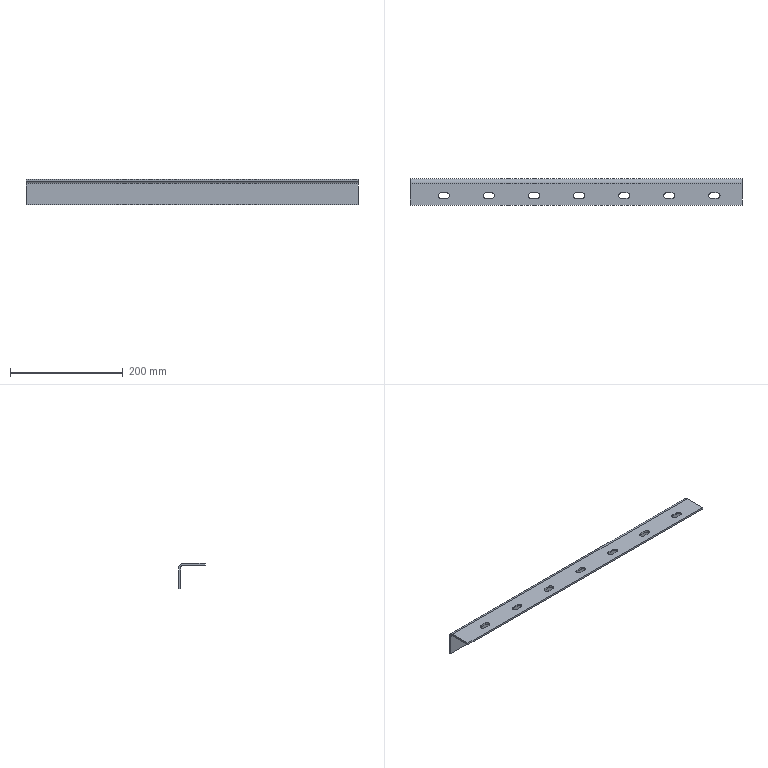Part | SolidWorks | features FlatPattern 1, ICE 1, SMBaseFlange 1, SheetMetal 1 | 1 solid | 49 faces | box 589 x 47 x 45 mm | volume 158032 mm3 | plane 26 | cylinder 23 | commonest cylinder face diameters 10 x22 16.4 x1
STEP:
#1=CARTESIAN_POINT('',(65.,-25.,-3.2));
#2=VERTEX_POINT('',#1);
#3=CARTESIAN_POINT('',(70.,-30.,-3.2));
#4=VERTEX_POINT('',#3);
#5=CARTESIAN_POINT('',(65.,-30.,-3.2));
#6=DIRECTION('',(0.,0.,-1.));
#7=DIRECTION('',(0.,1.,0.));
#8=AXIS2_PLACEMENT_3D('',#5,#6,#7);
#9=CIRCLE('',#8,5.);
#10=EDGE_CURVE('',#2,#4,#9,.T.);
#11=ORIENTED_EDGE('',*,*,#10,.T.);
#12=CARTESIAN_POINT('',(70.,-30.,0.));
#13=VERTEX_POINT('',#12);
#14=CARTESIAN_POINT('',(70.,-30.,-45.));
#15=DIRECTION('',(0.,0.,1.));
#16=VECTOR('',#15,1000.);
#17=LINE('',#14,#16);
#18=EDGE_CURVE('',#4,#13,#17,.T.);
#19=ORIENTED_EDGE('',*,*,#18,.T.);
#20=CARTESIAN_POINT('',(65.,-25.,0.));
#21=VERTEX_POINT('',#20);
#22=CARTESIAN_POINT('',(65.,-30.,0.));
#23=DIRECTION('',(0.,0.,1.));
#24=DIRECTION('',(1.,0.,0.));
#25=AXIS2_PLACEMENT_3D('',#22,#23,#24);
#26=CIRCLE('',#25,5.);
#27=EDGE_CURVE('',#13,#21,#26,.T.);
#28=ORIENTED_EDGE('',*,*,#27,.T.);
#29=CARTESIAN_POINT('',(65.,-25.,-45.));
#30=DIRECTION('',(0.,0.,1.));
#31=VECTOR('',#30,1000.);
#32=LINE('',#29,#31);
#33=EDGE_CURVE('',#2,#21,#32,.T.);
#34=ORIENTED_EDGE('',*,*,#33,.F.);
#35=EDGE_LOOP('',(#11,#19,#28,#34));
#36=FACE_OUTER_BOUND('',#35,.T.);
#37=CARTESIAN_POINT('',(65.,-30.,-45.));
#38=DIRECTION('',(0.,0.,1.));
#39=DIRECTION('',(1.,0.,0.));
#40=AXIS2_PLACEMENT_3D('',#37,#38,#39);
#41=CYLINDRICAL_SURFACE('',#40,5.);
#42=ADVANCED_FACE('',(#36),#41,.F.);
#43=CARTESIAN_POINT('',(145.,-25.,-3.2));
#44=VERTEX_POINT('',#43);
#45=CARTESIAN_POINT('',(150.,-30.,-3.2));
#46=VERTEX_POINT('',#45);
#47=CARTESIAN_POINT('',(145.,-30.,-3.2));
#48=DIRECTION('',(0.,0.,-1.));
#49=DIRECTION('',(0.,1.,0.));
#50=AXIS2_PLACEMENT_3D('',#47,#48,#49);
#51=CIRCLE('',#50,5.);
#52=EDGE_CURVE('',#44,#46,#51,.T.);
#53=ORIENTED_EDGE('',*,*,#52,.T.);
#54=CARTESIAN_POINT('',(150.,-30.,0.));
#55=VERTEX_POINT('',#54);
#56=CARTESIAN_POINT('',(150.,-30.,-45.));
#57=DIRECTION('',(0.,0.,1.));
#58=VECTOR('',#57,1000.);
#59=LINE('',#56,#58);
#60=EDGE_CURVE('',#46,#55,#59,.T.);
#61=ORIENTED_EDGE('',*,*,#60,.T.);
#62=CARTESIAN_POINT('',(145.,-25.,0.));
#63=VERTEX_POINT('',#62);
#64=CARTESIAN_POINT('',(145.,-30.,0.));
#65=DIRECTION('',(0.,0.,1.));
#66=DIRECTION('',(1.,0.,0.));
#67=AXIS2_PLACEMENT_3D('',#64,#65,#66);
#68=CIRCLE('',#67,5.);
#69=EDGE_CURVE('',#55,#63,#68,.T.);
#70=ORIENTED_EDGE('',*,*,#69,.T.);
#71=CARTESIAN_POINT('',(145.,-25.,-45.));
#72=DIRECTION('',(0.,0.,1.));
#73=VECTOR('',#72,1000.);
#74=LINE('',#71,#73);
#75=EDGE_CURVE('',#44,#63,#74,.T.);
#76=ORIENTED_EDGE('',*,*,#75,.F.);
#77=EDGE_LOOP('',(#53,#61,#70,#76));
#78=FACE_OUTER_BOUND('',#77,.T.);
#79=CARTESIAN_POINT('',(145.,-30.,-45.));
#80=DIRECTION('',(0.,0.,1.));
#81=DIRECTION('',(1.,0.,0.));
#82=AXIS2_PLACEMENT_3D('',#79,#80,#81);
#83=CYLINDRICAL_SURFACE('',#82,5.);
#84=ADVANCED_FACE('',(#78),#83,.F.);
#85=CARTESIAN_POINT('',(225.,-25.,-3.2));
#86=VERTEX_POINT('',#85);
#87=CARTESIAN_POINT('',(230.,-30.,-3.2));
#88=VERTEX_POINT('',#87);
#89=CARTESIAN_POINT('',(225.,-30.,-3.2));
#90=DIRECTION('',(0.,0.,-1.));
#91=DIRECTION('',(0.,1.,0.));
#92=AXIS2_PLACEMENT_3D('',#89,#90,#91);
#93=CIRCLE('',#92,5.);
#94=EDGE_CURVE('',#86,#88,#93,.T.);
#95=ORIENTED_EDGE('',*,*,#94,.T.);
#96=CARTESIAN_POINT('',(230.,-30.,0.));
#97=VERTEX_POINT('',#96);
#98=CARTESIAN_POINT('',(230.,-30.,-45.));
#99=DIRECTION('',(0.,0.,1.));
#100=VECTOR('',#99,1000.);
#101=LINE('',#98,#100);
#102=EDGE_CURVE('',#88,#97,#101,.T.);
#103=ORIENTED_EDGE('',*,*,#102,.T.);
#104=CARTESIAN_POINT('',(225.,-25.,0.));
#105=VERTEX_POINT('',#104);
#106=CARTESIAN_POINT('',(225.,-30.,0.));
#107=DIRECTION('',(0.,0.,1.));
#108=DIRECTION('',(1.,0.,0.));
#109=AXIS2_PLACEMENT_3D('',#106,#107,#108);
#110=CIRCLE('',#109,5.);
#111=EDGE_CURVE('',#97,#105,#110,.T.);
#112=ORIENTED_EDGE('',*,*,#111,.T.);
#113=CARTESIAN_POINT('',(225.,-25.,-45.));
#114=DIRECTION('',(0.,0.,1.));
#115=VECTOR('',#114,1000.);
#116=LINE('',#113,#115);
#117=EDGE_CURVE('',#86,#105,#116,.T.);
#118=ORIENTED_EDGE('',*,*,#117,.F.);
#119=EDGE_LOOP('',(#95,#103,#112,#118));
#120=FACE_OUTER_BOUND('',#119,.T.);
#121=CARTESIAN_POINT('',(225.,-30.,-45.));
#122=DIRECTION('',(0.,0.,1.));
#123=DIRECTION('',(1.,0.,0.));
#124=AXIS2_PLACEMENT_3D('',#121,#122,#123);
#125=CYLINDRICAL_SURFACE('',#124,5.);
#126=ADVANCED_FACE('',(#120),#125,.F.);
#127=CARTESIAN_POINT('',(305.,-25.,-3.2));
#128=VERTEX_POINT('',#127);
#129=CARTESIAN_POINT('',(310.,-30.,-3.2));
#130=VERTEX_POINT('',#129);
#131=CARTESIAN_POINT('',(305.,-30.,-3.2));
#132=DIRECTION('',(0.,0.,-1.));
#133=DIRECTION('',(0.,1.,0.));
#134=AXIS2_PLACEMENT_3D('',#131,#132,#133);
#135=CIRCLE('',#134,5.);
#136=EDGE_CURVE('',#128,#130,#135,.T.);
#137=ORIENTED_EDGE('',*,*,#136,.T.);
#138=CARTESIAN_POINT('',(310.,-30.,0.));
#139=VERTEX_POINT('',#138);
#140=CARTESIAN_POINT('',(310.,-30.,-45.));
#141=DIRECTION('',(0.,0.,1.));
#142=VECTOR('',#141,1000.);
#143=LINE('',#140,#142);
#144=EDGE_CURVE('',#130,#139,#143,.T.);
#145=ORIENTED_EDGE('',*,*,#144,.T.);
#146=CARTESIAN_POINT('',(305.,-25.,0.));
#147=VERTEX_POINT('',#146);
#148=CARTESIAN_POINT('',(305.,-30.,0.));
#149=DIRECTION('',(0.,0.,1.));
#150=DIRECTION('',(1.,0.,0.));
#151=AXIS2_PLACEMENT_3D('',#148,#149,#150);
#152=CIRCLE('',#151,5.);
#153=EDGE_CURVE('',#139,#147,#152,.T.);
#154=ORIENTED_EDGE('',*,*,#153,.T.);
#155=CARTESIAN_POINT('',(305.,-25.,-45.));
#156=DIRECTION('',(0.,0.,1.));
#157=VECTOR('',#156,1000.);
#158=LINE('',#155,#157);
#159=EDGE_CURVE('',#128,#147,#158,.T.);
#160=ORIENTED_EDGE('',*,*,#159,.F.);
#161=EDGE_LOOP('',(#137,#145,#154,#160));
#162=FACE_OUTER_BOUND('',#161,.T.);
#163=CARTESIAN_POINT('',(305.,-30.,-45.));
#164=DIRECTION('',(0.,0.,1.));
#165=DIRECTION('',(1.,0.,0.));
#166=AXIS2_PLACEMENT_3D('',#163,#164,#165);
#167=CYLINDRICAL_SURFACE('',#166,5.);
#168=ADVANCED_FACE('',(#162),#167,.F.);
#169=CARTESIAN_POINT('',(385.,-25.,-3.2));
#170=VERTEX_POINT('',#169);
#171=CARTESIAN_POINT('',(390.,-30.,-3.2));
#172=VERTEX_POINT('',#171);
#173=CARTESIAN_POINT('',(385.,-30.,-3.2));
#174=DIRECTION('',(0.,0.,-1.));
#175=DIRECTION('',(0.,1.,0.));
#176=AXIS2_PLACEMENT_3D('',#173,#174,#175);
#177=CIRCLE('',#176,5.);
#178=EDGE_CURVE('',#170,#172,#177,.T.);
#179=ORIENTED_EDGE('',*,*,#178,.T.);
#180=CARTESIAN_POINT('',(390.,-30.,0.));
#181=VERTEX_POINT('',#180);
#182=CARTESIAN_POINT('',(390.,-30.,-45.));
#183=DIRECTION('',(0.,0.,1.));
#184=VECTOR('',#183,1000.);
#185=LINE('',#182,#184);
#186=EDGE_CURVE('',#172,#181,#185,.T.);
#187=ORIENTED_EDGE('',*,*,#186,.T.);
#188=CARTESIAN_POINT('',(385.,-25.,0.));
#189=VERTEX_POINT('',#188);
#190=CARTESIAN_POINT('',(385.,-30.,0.));
#191=DIRECTION('',(0.,0.,1.));
#192=DIRECTION('',(1.,0.,0.));
#193=AXIS2_PLACEMENT_3D('',#190,#191,#192);
#194=CIRCLE('',#193,5.);
#195=EDGE_CURVE('',#181,#189,#194,.T.);
#196=ORIENTED_EDGE('',*,*,#195,.T.);
#197=CARTESIAN_POINT('',(385.,-25.,-45.));
#198=DIRECTION('',(0.,0.,1.));
#199=VECTOR('',#198,1000.);
#200=LINE('',#197,#199);
#201=EDGE_CURVE('',#170,#189,#200,.T.);
#202=ORIENTED_EDGE('',*,*,#201,.F.);
#203=EDGE_LOOP('',(#179,#187,#196,#202));
#204=FACE_OUTER_BOUND('',#203,.T.);
#205=CARTESIAN_POINT('',(385.,-30.,-45.));
#206=DIRECTION('',(0.,0.,1.));
#207=DIRECTION('',(1.,0.,0.));
#208=AXIS2_PLACEMENT_3D('',#205,#206,#207);
#209=CYLINDRICAL_SURFACE('',#208,5.);
#210=ADVANCED_FACE('',(#204),#209,.F.);
#211=CARTESIAN_POINT('',(465.,-25.,-3.2));
#212=VERTEX_POINT('',#211);
#213=CARTESIAN_POINT('',(470.,-30.,-3.2));
#214=VERTEX_POINT('',#213);
#215=CARTESIAN_POINT('',(465.,-30.,-3.2));
#216=DIRECTION('',(0.,0.,-1.));
#217=DIRECTION('',(0.,1.,0.));
#218=AXIS2_PLACEMENT_3D('',#215,#216,#217);
#219=CIRCLE('',#218,5.);
#220=EDGE_CURVE('',#212,#214,#219,.T.);
#221=ORIENTED_EDGE('',*,*,#220,.T.);
#222=CARTESIAN_POINT('',(470.,-30.,0.));
#223=VERTEX_POINT('',#222);
#224=CARTESIAN_POINT('',(470.,-30.,-45.));
#225=DIRECTION('',(0.,0.,1.));
#226=VECTOR('',#225,1000.);
#227=LINE('',#224,#226);
#228=EDGE_CURVE('',#214,#223,#227,.T.);
#229=ORIENTED_EDGE('',*,*,#228,.T.);
#230=CARTESIAN_POINT('',(465.,-25.,0.));
#231=VERTEX_POINT('',#230);
#232=CARTESIAN_POINT('',(465.,-30.,0.));
#233=DIRECTION('',(0.,0.,1.));
#234=DIRECTION('',(1.,0.,0.));
#235=AXIS2_PLACEMENT_3D('',#232,#233,#234);
#236=CIRCLE('',#235,5.);
#237=EDGE_CURVE('',#223,#231,#236,.T.);
#238=ORIENTED_EDGE('',*,*,#237,.T.);
#239=CARTESIAN_POINT('',(465.,-25.,-45.));
#240=DIRECTION('',(0.,0.,1.));
#241=VECTOR('',#240,1000.);
#242=LINE('',#239,#241);
#243=EDGE_CURVE('',#212,#231,#242,.T.);
#244=ORIENTED_EDGE('',*,*,#243,.F.);
#245=EDGE_LOOP('',(#221,#229,#238,#244));
#246=FACE_OUTER_BOUND('',#245,.T.);
#247=CARTESIAN_POINT('',(465.,-30.,-45.));
#248=DIRECTION('',(0.,0.,1.));
#249=DIRECTION('',(1.,0.,0.));
#250=AXIS2_PLACEMENT_3D('',#247,#248,#249);
#251=CYLINDRICAL_SURFACE('',#250,5.);
#252=ADVANCED_FACE('',(#246),#251,.F.);
#253=CARTESIAN_POINT('',(545.,-25.,-3.2));
#254=VERTEX_POINT('',#253);
#255=CARTESIAN_POINT('',(550.,-30.,-3.2));
#256=VERTEX_POINT('',#255);
#257=CARTESIAN_POINT('',(545.,-30.,-3.2));
#258=DIRECTION('',(0.,0.,-1.));
#259=DIRECTION('',(0.,1.,0.));
#260=AXIS2_PLACEMENT_3D('',#257,#258,#259);
#261=CIRCLE('',#260,5.);
#262=EDGE_CURVE('',#254,#256,#261,.T.);
#263=ORIENTED_EDGE('',*,*,#262,.T.);
#264=CARTESIAN_POINT('',(550.,-30.,0.));
#265=VERTEX_POINT('',#264);
#266=CARTESIAN_POINT('',(550.,-30.,-45.));
#267=DIRECTION('',(0.,0.,1.));
#268=VECTOR('',#267,1000.);
#269=LINE('',#266,#268);
#270=EDGE_CURVE('',#256,#265,#269,.T.);
#271=ORIENTED_EDGE('',*,*,#270,.T.);
#272=CARTESIAN_POINT('',(545.,-25.,0.));
#273=VERTEX_POINT('',#272);
#274=CARTESIAN_POINT('',(545.,-30.,0.));
#275=DIRECTION('',(0.,0.,1.));
#276=DIRECTION('',(1.,0.,0.));
#277=AXIS2_PLACEMENT_3D('',#274,#275,#276);
#278=CIRCLE('',#277,5.);
#279=EDGE_CURVE('',#265,#273,#278,.T.);
#280=ORIENTED_EDGE('',*,*,#279,.T.);
#281=CARTESIAN_POINT('',(545.,-25.,-45.));
#282=DIRECTION('',(0.,0.,1.));
#283=VECTOR('',#282,1000.);
#284=LINE('',#281,#283);
#285=EDGE_CURVE('',#254,#273,#284,.T.);
#286=ORIENTED_EDGE('',*,*,#285,.F.);
#287=EDGE_LOOP('',(#263,#271,#280,#286));
#288=FACE_OUTER_BOUND('',#287,.T.);
#289=CARTESIAN_POINT('',(545.,-30.,-45.));
#290=DIRECTION('',(0.,0.,1.));
#291=DIRECTION('',(1.,0.,0.));
#292=AXIS2_PLACEMENT_3D('',#289,#290,#291);
#293=CYLINDRICAL_SURFACE('',#292,5.);
#294=ADVANCED_FACE('',(#288),#293,.F.);
#295=CARTESIAN_POINT('',(589.,0.,-8.2));
#296=VERTEX_POINT('',#295);
#297=CARTESIAN_POINT('',(589.,-3.2,-8.2));
#298=VERTEX_POINT('',#297);
#299=CARTESIAN_POINT('',(589.,0.,-8.2));
#300=DIRECTION('',(0.,-1.,0.));
#301=VECTOR('',#300,1000.);
#302=LINE('',#299,#301);
#303=EDGE_CURVE('',#296,#298,#302,.T.);
#304=ORIENTED_EDGE('',*,*,#303,.F.);
#305=CARTESIAN_POINT('',(589.,-8.2,0.));
#306=VERTEX_POINT('',#305);
#307=CARTESIAN_POINT('',(589.,-8.2,-8.2));
#308=DIRECTION('',(1.,0.,0.));
#309=DIRECTION('',(0.,0.,1.));
#310=AXIS2_PLACEMENT_3D('',#307,#308,#309);
#311=CIRCLE('',#310,8.2);
#312=EDGE_CURVE('',#296,#306,#311,.T.);
#313=ORIENTED_EDGE('',*,*,#312,.T.);
#314=CARTESIAN_POINT('',(589.,-8.2,-3.2));
#315=VERTEX_POINT('',#314);
#316=CARTESIAN_POINT('',(589.,-8.2,-3.2));
#317=DIRECTION('',(0.,0.,1.));
#318=VECTOR('',#317,1000.);
#319=LINE('',#316,#318);
#320=EDGE_CURVE('',#315,#306,#319,.T.);
#321=ORIENTED_EDGE('',*,*,#320,.F.);
#322=CARTESIAN_POINT('',(589.,-8.2,-8.2));
#323=DIRECTION('',(1.,0.,0.));
#324=DIRECTION('',(0.,0.,-1.));
#325=AXIS2_PLACEMENT_3D('',#322,#323,#324);
#326=CIRCLE('',#325,5.);
#327=EDGE_CURVE('',#298,#315,#326,.T.);
#328=ORIENTED_EDGE('',*,*,#327,.F.);
#329=EDGE_LOOP('',(#304,#313,#321,#328));
#330=FACE_OUTER_BOUND('',#329,.T.);
#331=CARTESIAN_POINT('',(589.,0.,-8.2));
#332=DIRECTION('',(1.,0.,0.));
#333=DIRECTION('',(0.,0.,-1.));
#334=AXIS2_PLACEMENT_3D('',#331,#332,#333);
#335=PLANE('',#334);
#336=ADVANCED_FACE('',(#330),#335,.T.);
#337=CARTESIAN_POINT('',(589.,0.,-45.));
#338=VERTEX_POINT('',#337);
#339=CARTESIAN_POINT('',(589.,0.,0.));
#340=DIRECTION('',(0.,0.,1.));
#341=VECTOR('',#340,1000.);
#342=LINE('',#339,#341);
#343=EDGE_CURVE('',#338,#296,#342,.T.);
#344=ORIENTED_EDGE('',*,*,#343,.T.);
#345=ORIENTED_EDGE('',*,*,#303,.T.);
#346=CARTESIAN_POINT('',(589.,-3.2,-45.));
#347=VERTEX_POINT('',#346);
#348=CARTESIAN_POINT('',(589.,-3.2,0.));
#349=DIRECTION('',(0.,0.,1.));
#350=VECTOR('',#349,1000.);
#351=LINE('',#348,#350);
#352=EDGE_CURVE('',#347,#298,#351,.T.);
#353=ORIENTED_EDGE('',*,*,#352,.F.);
#354=CARTESIAN_POINT('',(589.,0.,-45.));
#355=DIRECTION('',(0.,-1.,0.));
#356=VECTOR('',#355,1000.);
#357=LINE('',#354,#356);
#358=EDGE_CURVE('',#338,#347,#357,.T.);
#359=ORIENTED_EDGE('',*,*,#358,.F.);
#360=EDGE_LOOP('',(#344,#345,#353,#359));
#361=FACE_OUTER_BOUND('',#360,.T.);
#362=CARTESIAN_POINT('',(589.,-8.2,-3.2));
#363=DIRECTION('',(1.,0.,0.));
#364=DIRECTION('',(0.,0.,-1.));
#365=AXIS2_PLACEMENT_3D('',#362,#363,#364);
#366=PLANE('',#365);
#367=ADVANCED_FACE('',(#361),#366,.T.);
#368=CARTESIAN_POINT('',(0.,-8.2,0.));
#369=VERTEX_POINT('',#368);
#370=CARTESIAN_POINT('',(0.,-8.2,-3.2));
#371=VERTEX_POINT('',#370);
#372=CARTESIAN_POINT('',(0.,-8.2,0.));
#373=DIRECTION('',(0.,0.,-1.));
#374=VECTOR('',#373,1000.);
#375=LINE('',#372,#374);
#376=EDGE_CURVE('',#369,#371,#375,.T.);
#377=ORIENTED_EDGE('',*,*,#376,.F.);
#378=CARTESIAN_POINT('',(0.,0.,-8.2));
#379=VERTEX_POINT('',#378);
#380=CARTESIAN_POINT('',(0.,-8.2,-8.2));
#381=DIRECTION('',(1.,0.,0.));
#382=DIRECTION('',(0.,0.,1.));
#383=AXIS2_PLACEMENT_3D('',#380,#381,#382);
#384=CIRCLE('',#383,8.2);
#385=EDGE_CURVE('',#379,#369,#384,.T.);
#386=ORIENTED_EDGE('',*,*,#385,.F.);
#387=CARTESIAN_POINT('',(0.,-3.2,-8.2));
#388=VERTEX_POINT('',#387);
#389=CARTESIAN_POINT('',(0.,-3.2,-8.2));
#390=DIRECTION('',(0.,1.,0.));
#391=VECTOR('',#390,1000.);
#392=LINE('',#389,#391);
#393=EDGE_CURVE('',#388,#379,#392,.T.);
#394=ORIENTED_EDGE('',*,*,#393,.F.);
#395=CARTESIAN_POINT('',(0.,-8.2,-8.2));
#396=DIRECTION('',(1.,0.,0.));
#397=DIRECTION('',(0.,0.,-1.));
#398=AXIS2_PLACEMENT_3D('',#395,#396,#397);
#399=CIRCLE('',#398,5.);
#400=EDGE_CURVE('',#388,#371,#399,.T.);
#401=ORIENTED_EDGE('',*,*,#400,.T.);
#402=EDGE_LOOP('',(#377,#386,#394,#401));
#403=FACE_OUTER_BOUND('',#402,.T.);
#404=CARTESIAN_POINT('',(0.,-8.2,0.));
#405=DIRECTION('',(-1.,0.,0.));
#406=DIRECTION('',(0.,0.,1.));
#407=AXIS2_PLACEMENT_3D('',#404,#405,#406);
#408=PLANE('',#407);
#409=ADVANCED_FACE('',(#403),#408,.T.);
#410=CARTESIAN_POINT('',(0.,-47.,0.));
#411=VERTEX_POINT('',#410);
#412=CARTESIAN_POINT('',(0.,0.,0.));
#413=DIRECTION('',(0.,-1.,0.));
#414=VECTOR('',#413,1000.);
#415=LINE('',#412,#414);
#416=EDGE_CURVE('',#369,#411,#415,.T.);
#417=ORIENTED_EDGE('',*,*,#416,.F.);
#418=ORIENTED_EDGE('',*,*,#376,.T.);
#419=CARTESIAN_POINT('',(0.,-47.,-3.2));
#420=VERTEX_POINT('',#419);
#421=CARTESIAN_POINT('',(0.,0.,-3.2));
#422=DIRECTION('',(0.,-1.,0.));
#423=VECTOR('',#422,1000.);
#424=LINE('',#421,#423);
#425=EDGE_CURVE('',#371,#420,#424,.T.);
#426=ORIENTED_EDGE('',*,*,#425,.T.);
#427=CARTESIAN_POINT('',(0.,-47.,-3.2));
#428=DIRECTION('',(0.,0.,1.));
#429=VECTOR('',#428,1000.);
#430=LINE('',#427,#429);
#431=EDGE_CURVE('',#420,#411,#430,.T.);
#432=ORIENTED_EDGE('',*,*,#431,.T.);
#433=EDGE_LOOP('',(#417,#418,#426,#432));
#434=FACE_OUTER_BOUND('',#433,.T.);
#435=CARTESIAN_POINT('',(0.,-3.2,-8.2));
#436=DIRECTION('',(-1.,0.,0.));
#437=DIRECTION('',(0.,0.,1.));
#438=AXIS2_PLACEMENT_3D('',#435,#436,#437);
#439=PLANE('',#438);
#440=ADVANCED_FACE('',(#434),#439,.T.);
#441=CARTESIAN_POINT('',(55.,-35.,0.));
#442=VERTEX_POINT('',#441);
#443=CARTESIAN_POINT('',(65.,-35.,0.));
#444=VERTEX_POINT('',#443);
#445=CARTESIAN_POINT('',(55.,-35.,0.));
#446=DIRECTION('',(1.,0.,0.));
#447=VECTOR('',#446,1000.);
#448=LINE('',#445,#447);
#449=EDGE_CURVE('',#442,#444,#448,.T.);
#450=ORIENTED_EDGE('',*,*,#449,.F.);
#451=CARTESIAN_POINT('',(55.,-25.,0.));
#452=VERTEX_POINT('',#451);
#453=CARTESIAN_POINT('',(55.,-30.,0.));
#454=DIRECTION('',(0.,0.,1.));
#455=DIRECTION('',(1.,0.,0.));
#456=AXIS2_PLACEMENT_3D('',#453,#454,#455);
#457=CIRCLE('',#456,5.);
#458=EDGE_CURVE('',#452,#442,#457,.T.);
#459=ORIENTED_EDGE('',*,*,#458,.F.);
#460=CARTESIAN_POINT('',(55.,-25.,0.));
#461=DIRECTION('',(-1.,0.,0.));
#462=VECTOR('',#461,1000.);
#463=LINE('',#460,#462);
#464=EDGE_CURVE('',#21,#452,#463,.T.);
#465=ORIENTED_EDGE('',*,*,#464,.F.);
#466=ORIENTED_EDGE('',*,*,#27,.F.);
#467=CARTESIAN_POINT('',(65.,-30.,0.));
#468=DIRECTION('',(0.,0.,1.));
#469=DIRECTION('',(1.,0.,0.));
#470=AXIS2_PLACEMENT_3D('',#467,#468,#469);
#471=CIRCLE('',#470,5.);
#472=EDGE_CURVE('',#444,#13,#471,.T.);
#473=ORIENTED_EDGE('',*,*,#472,.F.);
#474=EDGE_LOOP('',(#450,#459,#465,#466,#473));
#475=FACE_BOUND('',#474,.T.);
#476=CARTESIAN_POINT('',(135.,-35.,0.));
#477=VERTEX_POINT('',#476);
#478=CARTESIAN_POINT('',(145.,-35.,0.));
#479=VERTEX_POINT('',#478);
#480=CARTESIAN_POINT('',(135.,-35.,0.));
#481=DIRECTION('',(1.,0.,0.));
#482=VECTOR('',#481,1000.);
#483=LINE('',#480,#482);
#484=EDGE_CURVE('',#477,#479,#483,.T.);
#485=ORIENTED_EDGE('',*,*,#484,.F.);
#486=CARTESIAN_POINT('',(135.,-25.,0.));
#487=VERTEX_POINT('',#486);
#488=CARTESIAN_POINT('',(135.,-30.,0.));
#489=DIRECTION('',(0.,0.,1.));
#490=DIRECTION('',(1.,0.,0.));
#491=AXIS2_PLACEMENT_3D('',#488,#489,#490);
#492=CIRCLE('',#491,5.);
#493=EDGE_CURVE('',#487,#477,#492,.T.);
#494=ORIENTED_EDGE('',*,*,#493,.F.);
#495=CARTESIAN_POINT('',(135.,-25.,0.));
#496=DIRECTION('',(-1.,0.,0.));
#497=VECTOR('',#496,1000.);
#498=LINE('',#495,#497);
#499=EDGE_CURVE('',#63,#487,#498,.T.);
#500=ORIENTED_EDGE('',*,*,#499,.F.);
#501=ORIENTED_EDGE('',*,*,#69,.F.);
#502=CARTESIAN_POINT('',(145.,-30.,0.));
#503=DIRECTION('',(0.,0.,1.));
#504=DIRECTION('',(1.,0.,0.));
#505=AXIS2_PLACEMENT_3D('',#502,#503,#504);
#506=CIRCLE('',#505,5.);
#507=EDGE_CURVE('',#479,#55,#506,.T.);
#508=ORIENTED_EDGE('',*,*,#507,.F.);
#509=EDGE_LOOP('',(#485,#494,#500,#501,#508));
#510=FACE_BOUND('',#509,.T.);
#511=CARTESIAN_POINT('',(215.,-35.,0.));
#512=VERTEX_POINT('',#511);
#513=CARTESIAN_POINT('',(225.,-35.,0.));
#514=VERTEX_POINT('',#513);
#515=CARTESIAN_POINT('',(215.,-35.,0.));
#516=DIRECTION('',(1.,0.,0.));
#517=VECTOR('',#516,1000.);
#518=LINE('',#515,#517);
#519=EDGE_CURVE('',#512,#514,#518,.T.);
#520=ORIENTED_EDGE('',*,*,#519,.F.);
#521=CARTESIAN_POINT('',(215.,-25.,0.));
#522=VERTEX_POINT('',#521);
#523=CARTESIAN_POINT('',(215.,-30.,0.));
#524=DIRECTION('',(0.,0.,1.));
#525=DIRECTION('',(1.,0.,0.));
#526=AXIS2_PLACEMENT_3D('',#523,#524,#525);
#527=CIRCLE('',#526,5.);
#528=EDGE_CURVE('',#522,#512,#527,.T.);
#529=ORIENTED_EDGE('',*,*,#528,.F.);
#530=CARTESIAN_POINT('',(215.,-25.,0.));
#531=DIRECTION('',(-1.,0.,0.));
#532=VECTOR('',#531,1000.);
#533=LINE('',#530,#532);
#534=EDGE_CURVE('',#105,#522,#533,.T.);
#535=ORIENTED_EDGE('',*,*,#534,.F.);
#536=ORIENTED_EDGE('',*,*,#111,.F.);
#537=CARTESIAN_POINT('',(225.,-30.,0.));
#538=DIRECTION('',(0.,0.,1.));
#539=DIRECTION('',(1.,0.,0.));
#540=AXIS2_PLACEMENT_3D('',#537,#538,#539);
#541=CIRCLE('',#540,5.);
#542=EDGE_CURVE('',#514,#97,#541,.T.);
#543=ORIENTED_EDGE('',*,*,#542,.F.);
#544=EDGE_LOOP('',(#520,#529,#535,#536,#543));
#545=FACE_BOUND('',#544,.T.);
#546=CARTESIAN_POINT('',(295.,-35.,0.));
#547=VERTEX_POINT('',#546);
#548=CARTESIAN_POINT('',(305.,-35.,0.));
#549=VERTEX_POINT('',#548);
#550=CARTESIAN_POINT('',(295.,-35.,0.));
#551=DIRECTION('',(1.,0.,0.));
#552=VECTOR('',#551,1000.);
#553=LINE('',#550,#552);
#554=EDGE_CURVE('',#547,#549,#553,.T.);
#555=ORIENTED_EDGE('',*,*,#554,.F.);
#556=CARTESIAN_POINT('',(295.,-25.,0.));
#557=VERTEX_POINT('',#556);
#558=CARTESIAN_POINT('',(295.,-30.,0.));
#559=DIRECTION('',(0.,0.,1.));
#560=DIRECTION('',(1.,0.,0.));
#561=AXIS2_PLACEMENT_3D('',#558,#559,#560);
#562=CIRCLE('',#561,5.);
#563=EDGE_CURVE('',#557,#547,#562,.T.);
#564=ORIENTED_EDGE('',*,*,#563,.F.);
#565=CARTESIAN_POINT('',(295.,-25.,0.));
#566=DIRECTION('',(-1.,0.,0.));
#567=VECTOR('',#566,1000.);
#568=LINE('',#565,#567);
#569=EDGE_CURVE('',#147,#557,#568,.T.);
#570=ORIENTED_EDGE('',*,*,#569,.F.);
#571=ORIENTED_EDGE('',*,*,#153,.F.);
#572=CARTESIAN_POINT('',(305.,-30.,0.));
#573=DIRECTION('',(0.,0.,1.));
#574=DIRECTION('',(1.,0.,0.));
#575=AXIS2_PLACEMENT_3D('',#572,#573,#574);
#576=CIRCLE('',#575,5.);
#577=EDGE_CURVE('',#549,#139,#576,.T.);
#578=ORIENTED_EDGE('',*,*,#577,.F.);
#579=EDGE_LOOP('',(#555,#564,#570,#571,#578));
#580=FACE_BOUND('',#579,.T.);
#581=CARTESIAN_POINT('',(375.,-35.,0.));
#582=VERTEX_POINT('',#581);
#583=CARTESIAN_POINT('',(385.,-35.,0.));
#584=VERTEX_POINT('',#583);
#585=CARTESIAN_POINT('',(375.,-35.,0.));
#586=DIRECTION('',(1.,0.,0.));
#587=VECTOR('',#586,1000.);
#588=LINE('',#585,#587);
#589=EDGE_CURVE('',#582,#584,#588,.T.);
#590=ORIENTED_EDGE('',*,*,#589,.F.);
#591=CARTESIAN_POINT('',(375.,-25.,0.));
#592=VERTEX_POINT('',#591);
#593=CARTESIAN_POINT('',(375.,-30.,0.));
#594=DIRECTION('',(0.,0.,1.));
#595=DIRECTION('',(1.,0.,0.));
#596=AXIS2_PLACEMENT_3D('',#593,#594,#595);
#597=CIRCLE('',#596,5.);
#598=EDGE_CURVE('',#592,#582,#597,.T.);
#599=ORIENTED_EDGE('',*,*,#598,.F.);
#600=CARTESIAN_POINT('',(375.,-25.,0.));
#601=DIRECTION('',(-1.,0.,0.));
#602=VECTOR('',#601,1000.);
#603=LINE('',#600,#602);
#604=EDGE_CURVE('',#189,#592,#603,.T.);
#605=ORIENTED_EDGE('',*,*,#604,.F.);
#606=ORIENTED_EDGE('',*,*,#195,.F.);
#607=CARTESIAN_POINT('',(385.,-30.,0.));
#608=DIRECTION('',(0.,0.,1.));
#609=DIRECTION('',(1.,0.,0.));
#610=AXIS2_PLACEMENT_3D('',#607,#608,#609);
#611=CIRCLE('',#610,5.);
#612=EDGE_CURVE('',#584,#181,#611,.T.);
#613=ORIENTED_EDGE('',*,*,#612,.F.);
#614=EDGE_LOOP('',(#590,#599,#605,#606,#613));
#615=FACE_BOUND('',#614,.T.);
#616=CARTESIAN_POINT('',(455.,-35.,0.));
#617=VERTEX_POINT('',#616);
#618=CARTESIAN_POINT('',(465.,-35.,0.));
#619=VERTEX_POINT('',#618);
#620=CARTESIAN_POINT('',(455.,-35.,0.));
#621=DIRECTION('',(1.,0.,0.));
#622=VECTOR('',#621,1000.);
#623=LINE('',#620,#622);
#624=EDGE_CURVE('',#617,#619,#623,.T.);
#625=ORIENTED_EDGE('',*,*,#624,.F.);
#626=CARTESIAN_POINT('',(455.,-25.,0.));
#627=VERTEX_POINT('',#626);
#628=CARTESIAN_POINT('',(455.,-30.,0.));
#629=DIRECTION('',(0.,0.,1.));
#630=DIRECTION('',(1.,0.,0.));
#631=AXIS2_PLACEMENT_3D('',#628,#629,#630);
#632=CIRCLE('',#631,5.);
#633=EDGE_CURVE('',#627,#617,#632,.T.);
#634=ORIENTED_EDGE('',*,*,#633,.F.);
#635=CARTESIAN_POINT('',(455.,-25.,0.));
#636=DIRECTION('',(-1.,0.,0.));
#637=VECTOR('',#636,1000.);
#638=LINE('',#635,#637);
#639=EDGE_CURVE('',#231,#627,#638,.T.);
#640=ORIENTED_EDGE('',*,*,#639,.F.);
#641=ORIENTED_EDGE('',*,*,#237,.F.);
#642=CARTESIAN_POINT('',(465.,-30.,0.));
#643=DIRECTION('',(0.,0.,1.));
#644=DIRECTION('',(1.,0.,0.));
#645=AXIS2_PLACEMENT_3D('',#642,#643,#644);
#646=CIRCLE('',#645,5.);
#647=EDGE_CURVE('',#619,#223,#646,.T.);
#648=ORIENTED_EDGE('',*,*,#647,.F.);
#649=EDGE_LOOP('',(#625,#634,#640,#641,#648));
#650=FACE_BOUND('',#649,.T.);
#651=CARTESIAN_POINT('',(535.,-35.,0.));
#652=VERTEX_POINT('',#651);
#653=CARTESIAN_POINT('',(545.,-35.,0.));
#654=VERTEX_POINT('',#653);
#655=CARTESIAN_POINT('',(535.,-35.,0.));
#656=DIRECTION('',(1.,0.,0.));
#657=VECTOR('',#656,1000.);
#658=LINE('',#655,#657);
#659=EDGE_CURVE('',#652,#654,#658,.T.);
#660=ORIENTED_EDGE('',*,*,#659,.F.);
#661=CARTESIAN_POINT('',(535.,-25.,0.));
#662=VERTEX_POINT('',#661);
#663=CARTESIAN_POINT('',(535.,-30.,0.));
#664=DIRECTION('',(0.,0.,1.));
#665=DIRECTION('',(1.,0.,0.));
#666=AXIS2_PLACEMENT_3D('',#663,#664,#665);
#667=CIRCLE('',#666,5.);
#668=EDGE_CURVE('',#662,#652,#667,.T.);
#669=ORIENTED_EDGE('',*,*,#668,.F.);
#670=CARTESIAN_POINT('',(535.,-25.,0.));
#671=DIRECTION('',(-1.,0.,0.));
#672=VECTOR('',#671,1000.);
#673=LINE('',#670,#672);
#674=EDGE_CURVE('',#273,#662,#673,.T.);
#675=ORIENTED_EDGE('',*,*,#674,.F.);
#676=ORIENTED_EDGE('',*,*,#279,.F.);
#677=CARTESIAN_POINT('',(545.,-30.,0.));
#678=DIRECTION('',(0.,0.,1.));
#679=DIRECTION('',(1.,0.,0.));
#680=AXIS2_PLACEMENT_3D('',#677,#678,#679);
#681=CIRCLE('',#680,5.);
#682=EDGE_CURVE('',#654,#265,#681,.T.);
#683=ORIENTED_EDGE('',*,*,#682,.F.);
#684=EDGE_LOOP('',(#660,#669,#675,#676,#683));
#685=FACE_BOUND('',#684,.T.);
#686=ORIENTED_EDGE('',*,*,#416,.T.);
#687=CARTESIAN_POINT('',(589.,-47.,0.));
#688=VERTEX_POINT('',#687);
#689=CARTESIAN_POINT('',(589.,-47.,0.));
#690=DIRECTION('',(-1.,0.,0.));
#691=VECTOR('',#690,1000.);
#692=LINE('',#689,#691);
#693=EDGE_CURVE('',#688,#411,#692,.T.);
#694=ORIENTED_EDGE('',*,*,#693,.F.);
#695=CARTESIAN_POINT('',(589.,0.,0.));
#696=DIRECTION('',(0.,-1.,0.));
#697=VECTOR('',#696,1000.);
#698=LINE('',#695,#697);
#699=EDGE_CURVE('',#306,#688,#698,.T.);
#700=ORIENTED_EDGE('',*,*,#699,.F.);
#701=CARTESIAN_POINT('',(589.,-8.2,0.));
#702=DIRECTION('',(-1.,0.,0.));
#703=VECTOR('',#702,1000.);
#704=LINE('',#701,#703);
#705=EDGE_CURVE('',#306,#369,#704,.T.);
#706=ORIENTED_EDGE('',*,*,#705,.T.);
#707=EDGE_LOOP('',(#686,#694,#700,#706));
#708=FACE_OUTER_BOUND('',#707,.T.);
#709=CARTESIAN_POINT('',(589.,0.,0.));
#710=DIRECTION('',(0.,0.,-1.));
#711=DIRECTION('',(0.,1.,0.));
#712=AXIS2_PLACEMENT_3D('',#709,#710,#711);
#713=PLANE('',#712);
#714=ADVANCED_FACE('',(#475,#510,#545,#580,#615,#650,#685,#708),#713,.F.);
#715=ORIENTED_EDGE('',*,*,#431,.F.);
#716=CARTESIAN_POINT('',(589.,-47.,-3.2));
#717=VERTEX_POINT('',#716);
#718=CARTESIAN_POINT('',(589.,-47.,-3.2));
#719=DIRECTION('',(-1.,0.,0.));
#720=VECTOR('',#719,1000.);
#721=LINE('',#718,#720);
#722=EDGE_CURVE('',#717,#420,#721,.T.);
#723=ORIENTED_EDGE('',*,*,#722,.F.);
#724=CARTESIAN_POINT('',(589.,-47.,-3.2));
#725=DIRECTION('',(0.,0.,1.));
#726=VECTOR('',#725,1000.);
#727=LINE('',#724,#726);
#728=EDGE_CURVE('',#717,#688,#727,.T.);
#729=ORIENTED_EDGE('',*,*,#728,.T.);
#730=ORIENTED_EDGE('',*,*,#693,.T.);
#731=EDGE_LOOP('',(#715,#723,#729,#730));
#732=FACE_OUTER_BOUND('',#731,.T.);
#733=CARTESIAN_POINT('',(589.,-47.,-3.2));
#734=DIRECTION('',(0.,-1.,0.));
#735=DIRECTION('',(0.,0.,-1.));
#736=AXIS2_PLACEMENT_3D('',#733,#734,#735);
#737=PLANE('',#736);
#738=ADVANCED_FACE('',(#732),#737,.T.);
#739=CARTESIAN_POINT('',(55.,-35.,-3.2));
#740=VERTEX_POINT('',#739);
#741=CARTESIAN_POINT('',(55.,-25.,-3.2));
#742=VERTEX_POINT('',#741);
#743=CARTESIAN_POINT('',(55.,-30.,-3.2));
#744=DIRECTION('',(0.,0.,-1.));
#745=DIRECTION('',(0.,1.,0.));
#746=AXIS2_PLACEMENT_3D('',#743,#744,#745);
#747=CIRCLE('',#746,5.);
#748=EDGE_CURVE('',#740,#742,#747,.T.);
#749=ORIENTED_EDGE('',*,*,#748,.F.);
#750=CARTESIAN_POINT('',(65.,-35.,-3.2));
#751=VERTEX_POINT('',#750);
#752=CARTESIAN_POINT('',(589.,-35.,-3.2));
#753=DIRECTION('',(-1.,0.,0.));
#754=VECTOR('',#753,1000.);
#755=LINE('',#752,#754);
#756=EDGE_CURVE('',#751,#740,#755,.T.);
#757=ORIENTED_EDGE('',*,*,#756,.F.);
#758=CARTESIAN_POINT('',(65.,-30.,-3.2));
#759=DIRECTION('',(0.,0.,-1.));
#760=DIRECTION('',(0.,1.,0.));
#761=AXIS2_PLACEMENT_3D('',#758,#759,#760);
#762=CIRCLE('',#761,5.);
#763=EDGE_CURVE('',#4,#751,#762,.T.);
#764=ORIENTED_EDGE('',*,*,#763,.F.);
#765=ORIENTED_EDGE('',*,*,#10,.F.);
#766=CARTESIAN_POINT('',(589.,-25.,-3.2));
#767=DIRECTION('',(1.,0.,0.));
#768=VECTOR('',#767,1000.);
#769=LINE('',#766,#768);
#770=EDGE_CURVE('',#742,#2,#769,.T.);
#771=ORIENTED_EDGE('',*,*,#770,.F.);
#772=EDGE_LOOP('',(#749,#757,#764,#765,#771));
#773=FACE_BOUND('',#772,.T.);
#774=CARTESIAN_POINT('',(135.,-35.,-3.2));
#775=VERTEX_POINT('',#774);
#776=CARTESIAN_POINT('',(135.,-25.,-3.2));
#777=VERTEX_POINT('',#776);
#778=CARTESIAN_POINT('',(135.,-30.,-3.2));
#779=DIRECTION('',(0.,0.,-1.));
#780=DIRECTION('',(0.,1.,0.));
#781=AXIS2_PLACEMENT_3D('',#778,#779,#780);
#782=CIRCLE('',#781,5.);
#783=EDGE_CURVE('',#775,#777,#782,.T.);
#784=ORIENTED_EDGE('',*,*,#783,.F.);
#785=CARTESIAN_POINT('',(145.,-35.,-3.2));
#786=VERTEX_POINT('',#785);
#787=CARTESIAN_POINT('',(589.,-35.,-3.2));
#788=DIRECTION('',(-1.,0.,0.));
#789=VECTOR('',#788,1000.);
#790=LINE('',#787,#789);
#791=EDGE_CURVE('',#786,#775,#790,.T.);
#792=ORIENTED_EDGE('',*,*,#791,.F.);
#793=CARTESIAN_POINT('',(145.,-30.,-3.2));
#794=DIRECTION('',(0.,0.,-1.));
#795=DIRECTION('',(0.,1.,0.));
#796=AXIS2_PLACEMENT_3D('',#793,#794,#795);
#797=CIRCLE('',#796,5.);
#798=EDGE_CURVE('',#46,#786,#797,.T.);
#799=ORIENTED_EDGE('',*,*,#798,.F.);
#800=ORIENTED_EDGE('',*,*,#52,.F.);
#801=CARTESIAN_POINT('',(589.,-25.,-3.2));
#802=DIRECTION('',(1.,0.,0.));
#803=VECTOR('',#802,1000.);
#804=LINE('',#801,#803);
#805=EDGE_CURVE('',#777,#44,#804,.T.);
#806=ORIENTED_EDGE('',*,*,#805,.F.);
#807=EDGE_LOOP('',(#784,#792,#799,#800,#806));
#808=FACE_BOUND('',#807,.T.);
#809=CARTESIAN_POINT('',(215.,-35.,-3.2));
#810=VERTEX_POINT('',#809);
#811=CARTESIAN_POINT('',(215.,-25.,-3.2));
#812=VERTEX_POINT('',#811);
#813=CARTESIAN_POINT('',(215.,-30.,-3.2));
#814=DIRECTION('',(0.,0.,-1.));
#815=DIRECTION('',(0.,1.,0.));
#816=AXIS2_PLACEMENT_3D('',#813,#814,#815);
#817=CIRCLE('',#816,5.);
#818=EDGE_CURVE('',#810,#812,#817,.T.);
#819=ORIENTED_EDGE('',*,*,#818,.F.);
#820=CARTESIAN_POINT('',(225.,-35.,-3.2));
#821=VERTEX_POINT('',#820);
#822=CARTESIAN_POINT('',(589.,-35.,-3.2));
#823=DIRECTION('',(-1.,0.,0.));
#824=VECTOR('',#823,1000.);
#825=LINE('',#822,#824);
#826=EDGE_CURVE('',#821,#810,#825,.T.);
#827=ORIENTED_EDGE('',*,*,#826,.F.);
#828=CARTESIAN_POINT('',(225.,-30.,-3.2));
#829=DIRECTION('',(0.,0.,-1.));
#830=DIRECTION('',(0.,1.,0.));
#831=AXIS2_PLACEMENT_3D('',#828,#829,#830);
#832=CIRCLE('',#831,5.);
#833=EDGE_CURVE('',#88,#821,#832,.T.);
#834=ORIENTED_EDGE('',*,*,#833,.F.);
#835=ORIENTED_EDGE('',*,*,#94,.F.);
#836=CARTESIAN_POINT('',(589.,-25.,-3.2));
#837=DIRECTION('',(1.,0.,0.));
#838=VECTOR('',#837,1000.);
#839=LINE('',#836,#838);
#840=EDGE_CURVE('',#812,#86,#839,.T.);
#841=ORIENTED_EDGE('',*,*,#840,.F.);
#842=EDGE_LOOP('',(#819,#827,#834,#835,#841));
#843=FACE_BOUND('',#842,.T.);
#844=CARTESIAN_POINT('',(295.,-35.,-3.2));
#845=VERTEX_POINT('',#844);
#846=CARTESIAN_POINT('',(295.,-25.,-3.2));
#847=VERTEX_POINT('',#846);
#848=CARTESIAN_POINT('',(295.,-30.,-3.2));
#849=DIRECTION('',(0.,0.,-1.));
#850=DIRECTION('',(0.,1.,0.));
#851=AXIS2_PLACEMENT_3D('',#848,#849,#850);
#852=CIRCLE('',#851,5.);
#853=EDGE_CURVE('',#845,#847,#852,.T.);
#854=ORIENTED_EDGE('',*,*,#853,.F.);
#855=CARTESIAN_POINT('',(305.,-35.,-3.2));
#856=VERTEX_POINT('',#855);
#857=CARTESIAN_POINT('',(589.,-35.,-3.2));
#858=DIRECTION('',(-1.,0.,0.));
#859=VECTOR('',#858,1000.);
#860=LINE('',#857,#859);
#861=EDGE_CURVE('',#856,#845,#860,.T.);
#862=ORIENTED_EDGE('',*,*,#861,.F.);
#863=CARTESIAN_POINT('',(305.,-30.,-3.2));
#864=DIRECTION('',(0.,0.,-1.));
#865=DIRECTION('',(0.,1.,0.));
#866=AXIS2_PLACEMENT_3D('',#863,#864,#865);
#867=CIRCLE('',#866,5.);
#868=EDGE_CURVE('',#130,#856,#867,.T.);
#869=ORIENTED_EDGE('',*,*,#868,.F.);
#870=ORIENTED_EDGE('',*,*,#136,.F.);
#871=CARTESIAN_POINT('',(589.,-25.,-3.2));
#872=DIRECTION('',(1.,0.,0.));
#873=VECTOR('',#872,1000.);
#874=LINE('',#871,#873);
#875=EDGE_CURVE('',#847,#128,#874,.T.);
#876=ORIENTED_EDGE('',*,*,#875,.F.);
#877=EDGE_LOOP('',(#854,#862,#869,#870,#876));
#878=FACE_BOUND('',#877,.T.);
#879=CARTESIAN_POINT('',(375.,-35.,-3.2));
#880=VERTEX_POINT('',#879);
#881=CARTESIAN_POINT('',(375.,-25.,-3.2));
#882=VERTEX_POINT('',#881);
#883=CARTESIAN_POINT('',(375.,-30.,-3.2));
#884=DIRECTION('',(0.,0.,-1.));
#885=DIRECTION('',(0.,1.,0.));
#886=AXIS2_PLACEMENT_3D('',#883,#884,#885);
#887=CIRCLE('',#886,5.);
#888=EDGE_CURVE('',#880,#882,#887,.T.);
#889=ORIENTED_EDGE('',*,*,#888,.F.);
#890=CARTESIAN_POINT('',(385.,-35.,-3.2));
#891=VERTEX_POINT('',#890);
#892=CARTESIAN_POINT('',(589.,-35.,-3.2));
#893=DIRECTION('',(-1.,0.,0.));
#894=VECTOR('',#893,1000.);
#895=LINE('',#892,#894);
#896=EDGE_CURVE('',#891,#880,#895,.T.);
#897=ORIENTED_EDGE('',*,*,#896,.F.);
#898=CARTESIAN_POINT('',(385.,-30.,-3.2));
#899=DIRECTION('',(0.,0.,-1.));
#900=DIRECTION('',(0.,1.,0.));
#901=AXIS2_PLACEMENT_3D('',#898,#899,#900);
#902=CIRCLE('',#901,5.);
#903=EDGE_CURVE('',#172,#891,#902,.T.);
#904=ORIENTED_EDGE('',*,*,#903,.F.);
#905=ORIENTED_EDGE('',*,*,#178,.F.);
#906=CARTESIAN_POINT('',(589.,-25.,-3.2));
#907=DIRECTION('',(1.,0.,0.));
#908=VECTOR('',#907,1000.);
#909=LINE('',#906,#908);
#910=EDGE_CURVE('',#882,#170,#909,.T.);
#911=ORIENTED_EDGE('',*,*,#910,.F.);
#912=EDGE_LOOP('',(#889,#897,#904,#905,#911));
#913=FACE_BOUND('',#912,.T.);
#914=CARTESIAN_POINT('',(455.,-35.,-3.2));
#915=VERTEX_POINT('',#914);
#916=CARTESIAN_POINT('',(455.,-25.,-3.2));
#917=VERTEX_POINT('',#916);
#918=CARTESIAN_POINT('',(455.,-30.,-3.2));
#919=DIRECTION('',(0.,0.,-1.));
#920=DIRECTION('',(0.,1.,0.));
#921=AXIS2_PLACEMENT_3D('',#918,#919,#920);
#922=CIRCLE('',#921,5.);
#923=EDGE_CURVE('',#915,#917,#922,.T.);
#924=ORIENTED_EDGE('',*,*,#923,.F.);
#925=CARTESIAN_POINT('',(465.,-35.,-3.2));
#926=VERTEX_POINT('',#925);
#927=CARTESIAN_POINT('',(589.,-35.,-3.2));
#928=DIRECTION('',(-1.,0.,0.));
#929=VECTOR('',#928,1000.);
#930=LINE('',#927,#929);
#931=EDGE_CURVE('',#926,#915,#930,.T.);
#932=ORIENTED_EDGE('',*,*,#931,.F.);
#933=CARTESIAN_POINT('',(465.,-30.,-3.2));
#934=DIRECTION('',(0.,0.,-1.));
#935=DIRECTION('',(0.,1.,0.));
#936=AXIS2_PLACEMENT_3D('',#933,#934,#935);
#937=CIRCLE('',#936,5.);
#938=EDGE_CURVE('',#214,#926,#937,.T.);
#939=ORIENTED_EDGE('',*,*,#938,.F.);
#940=ORIENTED_EDGE('',*,*,#220,.F.);
#941=CARTESIAN_POINT('',(589.,-25.,-3.2));
#942=DIRECTION('',(1.,0.,0.));
#943=VECTOR('',#942,1000.);
#944=LINE('',#941,#943);
#945=EDGE_CURVE('',#917,#212,#944,.T.);
#946=ORIENTED_EDGE('',*,*,#945,.F.);
#947=EDGE_LOOP('',(#924,#932,#939,#940,#946));
#948=FACE_BOUND('',#947,.T.);
#949=CARTESIAN_POINT('',(535.,-35.,-3.2));
#950=VERTEX_POINT('',#949);
#951=CARTESIAN_POINT('',(535.,-25.,-3.2));
#952=VERTEX_POINT('',#951);
#953=CARTESIAN_POINT('',(535.,-30.,-3.2));
#954=DIRECTION('',(0.,0.,-1.));
#955=DIRECTION('',(0.,1.,0.));
#956=AXIS2_PLACEMENT_3D('',#953,#954,#955);
#957=CIRCLE('',#956,5.);
#958=EDGE_CURVE('',#950,#952,#957,.T.);
#959=ORIENTED_EDGE('',*,*,#958,.F.);
#960=CARTESIAN_POINT('',(545.,-35.,-3.2));
#961=VERTEX_POINT('',#960);
#962=CARTESIAN_POINT('',(589.,-35.,-3.2));
#963=DIRECTION('',(-1.,0.,0.));
#964=VECTOR('',#963,1000.);
#965=LINE('',#962,#964);
#966=EDGE_CURVE('',#961,#950,#965,.T.);
#967=ORIENTED_EDGE('',*,*,#966,.F.);
#968=CARTESIAN_POINT('',(545.,-30.,-3.2));
#969=DIRECTION('',(0.,0.,-1.));
#970=DIRECTION('',(0.,1.,0.));
#971=AXIS2_PLACEMENT_3D('',#968,#969,#970);
#972=CIRCLE('',#971,5.);
#973=EDGE_CURVE('',#256,#961,#972,.T.);
#974=ORIENTED_EDGE('',*,*,#973,.F.);
#975=ORIENTED_EDGE('',*,*,#262,.F.);
#976=CARTESIAN_POINT('',(589.,-25.,-3.2));
#977=DIRECTION('',(1.,0.,0.));
#978=VECTOR('',#977,1000.);
#979=LINE('',#976,#978);
#980=EDGE_CURVE('',#952,#254,#979,.T.);
#981=ORIENTED_EDGE('',*,*,#980,.F.);
#982=EDGE_LOOP('',(#959,#967,#974,#975,#981));
#983=FACE_BOUND('',#982,.T.);
#984=ORIENTED_EDGE('',*,*,#425,.F.);
#985=CARTESIAN_POINT('',(589.,-8.2,-3.2));
#986=DIRECTION('',(-1.,0.,0.));
#987=VECTOR('',#986,1000.);
#988=LINE('',#985,#987);
#989=EDGE_CURVE('',#315,#371,#988,.T.);
#990=ORIENTED_EDGE('',*,*,#989,.F.);
#991=CARTESIAN_POINT('',(589.,0.,-3.2));
#992=DIRECTION('',(0.,-1.,0.));
#993=VECTOR('',#992,1000.);
#994=LINE('',#991,#993);
#995=EDGE_CURVE('',#315,#717,#994,.T.);
#996=ORIENTED_EDGE('',*,*,#995,.T.);
#997=ORIENTED_EDGE('',*,*,#722,.T.);
#998=EDGE_LOOP('',(#984,#990,#996,#997));
#999=FACE_OUTER_BOUND('',#998,.T.);
#1000=CARTESIAN_POINT('',(589.,0.,-3.2));
#1001=DIRECTION('',(0.,0.,-1.));
#1002=DIRECTION('',(0.,1.,0.));
#1003=AXIS2_PLACEMENT_3D('',#1000,#1001,#1002);
#1004=PLANE('',#1003);
#1005=ADVANCED_FACE('',(#773,#808,#843,#878,#913,#948,#983,#999),#1004,.T.);
#1006=ORIENTED_EDGE('',*,*,#400,.F.);
#1007=CARTESIAN_POINT('',(589.,-3.2,-8.2));
#1008=DIRECTION('',(-1.,0.,0.));
#1009=VECTOR('',#1008,1000.);
#1010=LINE('',#1007,#1009);
#1011=EDGE_CURVE('',#298,#388,#1010,.T.);
#1012=ORIENTED_EDGE('',*,*,#1011,.F.);
#1013=ORIENTED_EDGE('',*,*,#327,.T.);
#1014=ORIENTED_EDGE('',*,*,#989,.T.);
#1015=EDGE_LOOP('',(#1006,#1012,#1013,#1014));
#1016=FACE_OUTER_BOUND('',#1015,.T.);
#1017=CARTESIAN_POINT('',(589.,-8.2,-8.2));
#1018=DIRECTION('',(-1.,0.,0.));
#1019=DIRECTION('',(0.,0.,1.));
#1020=AXIS2_PLACEMENT_3D('',#1017,#1018,#1019);
#1021=CYLINDRICAL_SURFACE('',#1020,5.);
#1022=ADVANCED_FACE('',(#1016),#1021,.F.);
#1023=CARTESIAN_POINT('',(0.,-3.2,-45.));
#1024=VERTEX_POINT('',#1023);
#1025=CARTESIAN_POINT('',(0.,-3.2,0.));
#1026=DIRECTION('',(0.,0.,1.));
#1027=VECTOR('',#1026,1000.);
#1028=LINE('',#1025,#1027);
#1029=EDGE_CURVE('',#1024,#388,#1028,.T.);
#1030=ORIENTED_EDGE('',*,*,#1029,.F.);
#1031=CARTESIAN_POINT('',(589.,-3.2,-45.));
#1032=DIRECTION('',(-1.,0.,0.));
#1033=VECTOR('',#1032,1000.);
#1034=LINE('',#1031,#1033);
#1035=EDGE_CURVE('',#347,#1024,#1034,.T.);
#1036=ORIENTED_EDGE('',*,*,#1035,.F.);
#1037=ORIENTED_EDGE('',*,*,#352,.T.);
#1038=ORIENTED_EDGE('',*,*,#1011,.T.);
#1039=EDGE_LOOP('',(#1030,#1036,#1037,#1038));
#1040=FACE_OUTER_BOUND('',#1039,.T.);
#1041=CARTESIAN_POINT('',(589.,-3.2,0.));
#1042=DIRECTION('',(0.,-1.,0.));
#1043=DIRECTION('',(0.,0.,-1.));
#1044=AXIS2_PLACEMENT_3D('',#1041,#1042,#1043);
#1045=PLANE('',#1044);
#1046=ADVANCED_FACE('',(#1040),#1045,.T.);
#1047=CARTESIAN_POINT('',(0.,0.,-45.));
#1048=VERTEX_POINT('',#1047);
#1049=CARTESIAN_POINT('',(0.,0.,-45.));
#1050=DIRECTION('',(0.,-1.,0.));
#1051=VECTOR('',#1050,1000.);
#1052=LINE('',#1049,#1051);
#1053=EDGE_CURVE('',#1048,#1024,#1052,.T.);
#1054=ORIENTED_EDGE('',*,*,#1053,.F.);
#1055=CARTESIAN_POINT('',(589.,0.,-45.));
#1056=DIRECTION('',(-1.,0.,0.));
#1057=VECTOR('',#1056,1000.);
#1058=LINE('',#1055,#1057);
#1059=EDGE_CURVE('',#338,#1048,#1058,.T.);
#1060=ORIENTED_EDGE('',*,*,#1059,.F.);
#1061=ORIENTED_EDGE('',*,*,#358,.T.);
#1062=ORIENTED_EDGE('',*,*,#1035,.T.);
#1063=EDGE_LOOP('',(#1054,#1060,#1061,#1062));
#1064=FACE_OUTER_BOUND('',#1063,.T.);
#1065=CARTESIAN_POINT('',(589.,0.,-45.));
#1066=DIRECTION('',(0.,0.,-1.));
#1067=DIRECTION('',(0.,1.,0.));
#1068=AXIS2_PLACEMENT_3D('',#1065,#1066,#1067);
#1069=PLANE('',#1068);
#1070=ADVANCED_FACE('',(#1064),#1069,.T.);
#1071=CARTESIAN_POINT('',(0.,0.,0.));
#1072=DIRECTION('',(0.,0.,1.));
#1073=VECTOR('',#1072,1000.);
#1074=LINE('',#1071,#1073);
#1075=EDGE_CURVE('',#1048,#379,#1074,.T.);
#1076=ORIENTED_EDGE('',*,*,#1075,.T.);
#1077=CARTESIAN_POINT('',(589.,0.,-8.2));
#1078=DIRECTION('',(-1.,0.,0.));
#1079=VECTOR('',#1078,1000.);
#1080=LINE('',#1077,#1079);
#1081=EDGE_CURVE('',#296,#379,#1080,.T.);
#1082=ORIENTED_EDGE('',*,*,#1081,.F.);
#1083=ORIENTED_EDGE('',*,*,#343,.F.);
#1084=ORIENTED_EDGE('',*,*,#1059,.T.);
#1085=EDGE_LOOP('',(#1076,#1082,#1083,#1084));
#1086=FACE_OUTER_BOUND('',#1085,.T.);
#1087=CARTESIAN_POINT('',(589.,0.,0.));
#1088=DIRECTION('',(0.,-1.,0.));
#1089=DIRECTION('',(0.,0.,-1.));
#1090=AXIS2_PLACEMENT_3D('',#1087,#1088,#1089);
#1091=PLANE('',#1090);
#1092=ADVANCED_FACE('',(#1086),#1091,.F.);
#1093=ORIENTED_EDGE('',*,*,#385,.T.);
#1094=ORIENTED_EDGE('',*,*,#705,.F.);
#1095=ORIENTED_EDGE('',*,*,#312,.F.);
#1096=ORIENTED_EDGE('',*,*,#1081,.T.);
#1097=EDGE_LOOP('',(#1093,#1094,#1095,#1096));
#1098=FACE_OUTER_BOUND('',#1097,.T.);
#1099=CARTESIAN_POINT('',(589.,-8.2,-8.2));
#1100=DIRECTION('',(-1.,0.,0.));
#1101=DIRECTION('',(0.,0.,1.));
#1102=AXIS2_PLACEMENT_3D('',#1099,#1100,#1101);
#1103=CYLINDRICAL_SURFACE('',#1102,8.2);
#1104=ADVANCED_FACE('',(#1098),#1103,.T.);
#1105=ORIENTED_EDGE('',*,*,#699,.T.);
#1106=ORIENTED_EDGE('',*,*,#728,.F.);
#1107=ORIENTED_EDGE('',*,*,#995,.F.);
#1108=ORIENTED_EDGE('',*,*,#320,.T.);
#1109=EDGE_LOOP('',(#1105,#1106,#1107,#1108));
#1110=FACE_OUTER_BOUND('',#1109,.T.);
#1111=CARTESIAN_POINT('',(589.,-8.2,-8.2));
#1112=DIRECTION('',(1.,0.,0.));
#1113=DIRECTION('',(0.,0.,-1.));
#1114=AXIS2_PLACEMENT_3D('',#1111,#1112,#1113);
#1115=PLANE('',#1114);
#1116=ADVANCED_FACE('',(#1110),#1115,.T.);
#1117=ORIENTED_EDGE('',*,*,#1029,.T.);
#1118=ORIENTED_EDGE('',*,*,#393,.T.);
#1119=ORIENTED_EDGE('',*,*,#1075,.F.);
#1120=ORIENTED_EDGE('',*,*,#1053,.T.);
#1121=EDGE_LOOP('',(#1117,#1118,#1119,#1120));
#1122=FACE_OUTER_BOUND('',#1121,.T.);
#1123=CARTESIAN_POINT('',(0.,-8.2,-8.2));
#1124=DIRECTION('',(1.,0.,0.));
#1125=DIRECTION('',(0.,0.,-1.));
#1126=AXIS2_PLACEMENT_3D('',#1123,#1124,#1125);
#1127=PLANE('',#1126);
#1128=ADVANCED_FACE('',(#1122),#1127,.F.);
#1129=ORIENTED_EDGE('',*,*,#958,.T.);
#1130=CARTESIAN_POINT('',(535.,-25.,-45.));
#1131=DIRECTION('',(0.,0.,1.));
#1132=VECTOR('',#1131,1000.);
#1133=LINE('',#1130,#1132);
#1134=EDGE_CURVE('',#952,#662,#1133,.T.);
#1135=ORIENTED_EDGE('',*,*,#1134,.T.);
#1136=ORIENTED_EDGE('',*,*,#668,.T.);
#1137=CARTESIAN_POINT('',(535.,-35.,-45.));
#1138=DIRECTION('',(0.,0.,1.));
#1139=VECTOR('',#1138,1000.);
#1140=LINE('',#1137,#1139);
#1141=EDGE_CURVE('',#950,#652,#1140,.T.);
#1142=ORIENTED_EDGE('',*,*,#1141,.F.);
#1143=EDGE_LOOP('',(#1129,#1135,#1136,#1142));
#1144=FACE_OUTER_BOUND('',#1143,.T.);
#1145=CARTESIAN_POINT('',(535.,-30.,-45.));
#1146=DIRECTION('',(0.,0.,1.));
#1147=DIRECTION('',(1.,0.,0.));
#1148=AXIS2_PLACEMENT_3D('',#1145,#1146,#1147);
#1149=CYLINDRICAL_SURFACE('',#1148,5.);
#1150=ADVANCED_FACE('',(#1144),#1149,.F.);
#1151=ORIENTED_EDGE('',*,*,#980,.T.);
#1152=ORIENTED_EDGE('',*,*,#285,.T.);
#1153=ORIENTED_EDGE('',*,*,#674,.T.);
#1154=ORIENTED_EDGE('',*,*,#1134,.F.);
#1155=EDGE_LOOP('',(#1151,#1152,#1153,#1154));
#1156=FACE_OUTER_BOUND('',#1155,.T.);
#1157=CARTESIAN_POINT('',(535.,-25.,-45.));
#1158=DIRECTION('',(0.,1.,0.));
#1159=DIRECTION('',(0.,0.,1.));
#1160=AXIS2_PLACEMENT_3D('',#1157,#1158,#1159);
#1161=PLANE('',#1160);
#1162=ADVANCED_FACE('',(#1156),#1161,.F.);
#1163=ORIENTED_EDGE('',*,*,#270,.F.);
#1164=ORIENTED_EDGE('',*,*,#973,.T.);
#1165=CARTESIAN_POINT('',(545.,-35.,-45.));
#1166=DIRECTION('',(0.,0.,1.));
#1167=VECTOR('',#1166,1000.);
#1168=LINE('',#1165,#1167);
#1169=EDGE_CURVE('',#961,#654,#1168,.T.);
#1170=ORIENTED_EDGE('',*,*,#1169,.T.);
#1171=ORIENTED_EDGE('',*,*,#682,.T.);
#1172=EDGE_LOOP('',(#1163,#1164,#1170,#1171));
#1173=FACE_OUTER_BOUND('',#1172,.T.);
#1174=CARTESIAN_POINT('',(545.,-30.,-45.));
#1175=DIRECTION('',(0.,0.,1.));
#1176=DIRECTION('',(1.,0.,0.));
#1177=AXIS2_PLACEMENT_3D('',#1174,#1175,#1176);
#1178=CYLINDRICAL_SURFACE('',#1177,5.);
#1179=ADVANCED_FACE('',(#1173),#1178,.F.);
#1180=ORIENTED_EDGE('',*,*,#966,.T.);
#1181=ORIENTED_EDGE('',*,*,#1141,.T.);
#1182=ORIENTED_EDGE('',*,*,#659,.T.);
#1183=ORIENTED_EDGE('',*,*,#1169,.F.);
#1184=EDGE_LOOP('',(#1180,#1181,#1182,#1183));
#1185=FACE_OUTER_BOUND('',#1184,.T.);
#1186=CARTESIAN_POINT('',(535.,-35.,-45.));
#1187=DIRECTION('',(0.,-1.,0.));
#1188=DIRECTION('',(0.,0.,-1.));
#1189=AXIS2_PLACEMENT_3D('',#1186,#1187,#1188);
#1190=PLANE('',#1189);
#1191=ADVANCED_FACE('',(#1185),#1190,.F.);
#1192=ORIENTED_EDGE('',*,*,#923,.T.);
#1193=CARTESIAN_POINT('',(455.,-25.,-45.));
#1194=DIRECTION('',(0.,0.,1.));
#1195=VECTOR('',#1194,1000.);
#1196=LINE('',#1193,#1195);
#1197=EDGE_CURVE('',#917,#627,#1196,.T.);
#1198=ORIENTED_EDGE('',*,*,#1197,.T.);
#1199=ORIENTED_EDGE('',*,*,#633,.T.);
#1200=CARTESIAN_POINT('',(455.,-35.,-45.));
#1201=DIRECTION('',(0.,0.,1.));
#1202=VECTOR('',#1201,1000.);
#1203=LINE('',#1200,#1202);
#1204=EDGE_CURVE('',#915,#617,#1203,.T.);
#1205=ORIENTED_EDGE('',*,*,#1204,.F.);
#1206=EDGE_LOOP('',(#1192,#1198,#1199,#1205));
#1207=FACE_OUTER_BOUND('',#1206,.T.);
#1208=CARTESIAN_POINT('',(455.,-30.,-45.));
#1209=DIRECTION('',(0.,0.,1.));
#1210=DIRECTION('',(1.,0.,0.));
#1211=AXIS2_PLACEMENT_3D('',#1208,#1209,#1210);
#1212=CYLINDRICAL_SURFACE('',#1211,5.);
#1213=ADVANCED_FACE('',(#1207),#1212,.F.);
#1214=ORIENTED_EDGE('',*,*,#945,.T.);
#1215=ORIENTED_EDGE('',*,*,#243,.T.);
#1216=ORIENTED_EDGE('',*,*,#639,.T.);
#1217=ORIENTED_EDGE('',*,*,#1197,.F.);
#1218=EDGE_LOOP('',(#1214,#1215,#1216,#1217));
#1219=FACE_OUTER_BOUND('',#1218,.T.);
#1220=CARTESIAN_POINT('',(455.,-25.,-45.));
#1221=DIRECTION('',(0.,1.,0.));
#1222=DIRECTION('',(0.,0.,1.));
#1223=AXIS2_PLACEMENT_3D('',#1220,#1221,#1222);
#1224=PLANE('',#1223);
#1225=ADVANCED_FACE('',(#1219),#1224,.F.);
#1226=ORIENTED_EDGE('',*,*,#228,.F.);
#1227=ORIENTED_EDGE('',*,*,#938,.T.);
#1228=CARTESIAN_POINT('',(465.,-35.,-45.));
#1229=DIRECTION('',(0.,0.,1.));
#1230=VECTOR('',#1229,1000.);
#1231=LINE('',#1228,#1230);
#1232=EDGE_CURVE('',#926,#619,#1231,.T.);
#1233=ORIENTED_EDGE('',*,*,#1232,.T.);
#1234=ORIENTED_EDGE('',*,*,#647,.T.);
#1235=EDGE_LOOP('',(#1226,#1227,#1233,#1234));
#1236=FACE_OUTER_BOUND('',#1235,.T.);
#1237=CARTESIAN_POINT('',(465.,-30.,-45.));
#1238=DIRECTION('',(0.,0.,1.));
#1239=DIRECTION('',(1.,0.,0.));
#1240=AXIS2_PLACEMENT_3D('',#1237,#1238,#1239);
#1241=CYLINDRICAL_SURFACE('',#1240,5.);
#1242=ADVANCED_FACE('',(#1236),#1241,.F.);
#1243=ORIENTED_EDGE('',*,*,#931,.T.);
#1244=ORIENTED_EDGE('',*,*,#1204,.T.);
#1245=ORIENTED_EDGE('',*,*,#624,.T.);
#1246=ORIENTED_EDGE('',*,*,#1232,.F.);
#1247=EDGE_LOOP('',(#1243,#1244,#1245,#1246));
#1248=FACE_OUTER_BOUND('',#1247,.T.);
#1249=CARTESIAN_POINT('',(455.,-35.,-45.));
#1250=DIRECTION('',(0.,-1.,0.));
#1251=DIRECTION('',(0.,0.,-1.));
#1252=AXIS2_PLACEMENT_3D('',#1249,#1250,#1251);
#1253=PLANE('',#1252);
#1254=ADVANCED_FACE('',(#1248),#1253,.F.);
#1255=ORIENTED_EDGE('',*,*,#888,.T.);
#1256=CARTESIAN_POINT('',(375.,-25.,-45.));
#1257=DIRECTION('',(0.,0.,1.));
#1258=VECTOR('',#1257,1000.);
#1259=LINE('',#1256,#1258);
#1260=EDGE_CURVE('',#882,#592,#1259,.T.);
#1261=ORIENTED_EDGE('',*,*,#1260,.T.);
#1262=ORIENTED_EDGE('',*,*,#598,.T.);
#1263=CARTESIAN_POINT('',(375.,-35.,-45.));
#1264=DIRECTION('',(0.,0.,1.));
#1265=VECTOR('',#1264,1000.);
#1266=LINE('',#1263,#1265);
#1267=EDGE_CURVE('',#880,#582,#1266,.T.);
#1268=ORIENTED_EDGE('',*,*,#1267,.F.);
#1269=EDGE_LOOP('',(#1255,#1261,#1262,#1268));
#1270=FACE_OUTER_BOUND('',#1269,.T.);
#1271=CARTESIAN_POINT('',(375.,-30.,-45.));
#1272=DIRECTION('',(0.,0.,1.));
#1273=DIRECTION('',(1.,0.,0.));
#1274=AXIS2_PLACEMENT_3D('',#1271,#1272,#1273);
#1275=CYLINDRICAL_SURFACE('',#1274,5.);
#1276=ADVANCED_FACE('',(#1270),#1275,.F.);
#1277=ORIENTED_EDGE('',*,*,#910,.T.);
#1278=ORIENTED_EDGE('',*,*,#201,.T.);
#1279=ORIENTED_EDGE('',*,*,#604,.T.);
#1280=ORIENTED_EDGE('',*,*,#1260,.F.);
#1281=EDGE_LOOP('',(#1277,#1278,#1279,#1280));
#1282=FACE_OUTER_BOUND('',#1281,.T.);
#1283=CARTESIAN_POINT('',(375.,-25.,-45.));
#1284=DIRECTION('',(0.,1.,0.));
#1285=DIRECTION('',(0.,0.,1.));
#1286=AXIS2_PLACEMENT_3D('',#1283,#1284,#1285);
#1287=PLANE('',#1286);
#1288=ADVANCED_FACE('',(#1282),#1287,.F.);
#1289=ORIENTED_EDGE('',*,*,#186,.F.);
#1290=ORIENTED_EDGE('',*,*,#903,.T.);
#1291=CARTESIAN_POINT('',(385.,-35.,-45.));
#1292=DIRECTION('',(0.,0.,1.));
#1293=VECTOR('',#1292,1000.);
#1294=LINE('',#1291,#1293);
#1295=EDGE_CURVE('',#891,#584,#1294,.T.);
#1296=ORIENTED_EDGE('',*,*,#1295,.T.);
#1297=ORIENTED_EDGE('',*,*,#612,.T.);
#1298=EDGE_LOOP('',(#1289,#1290,#1296,#1297));
#1299=FACE_OUTER_BOUND('',#1298,.T.);
#1300=CARTESIAN_POINT('',(385.,-30.,-45.));
#1301=DIRECTION('',(0.,0.,1.));
#1302=DIRECTION('',(1.,0.,0.));
#1303=AXIS2_PLACEMENT_3D('',#1300,#1301,#1302);
#1304=CYLINDRICAL_SURFACE('',#1303,5.);
#1305=ADVANCED_FACE('',(#1299),#1304,.F.);
#1306=ORIENTED_EDGE('',*,*,#896,.T.);
#1307=ORIENTED_EDGE('',*,*,#1267,.T.);
#1308=ORIENTED_EDGE('',*,*,#589,.T.);
#1309=ORIENTED_EDGE('',*,*,#1295,.F.);
#1310=EDGE_LOOP('',(#1306,#1307,#1308,#1309));
#1311=FACE_OUTER_BOUND('',#1310,.T.);
#1312=CARTESIAN_POINT('',(375.,-35.,-45.));
#1313=DIRECTION('',(0.,-1.,0.));
#1314=DIRECTION('',(0.,0.,-1.));
#1315=AXIS2_PLACEMENT_3D('',#1312,#1313,#1314);
#1316=PLANE('',#1315);
#1317=ADVANCED_FACE('',(#1311),#1316,.F.);
#1318=ORIENTED_EDGE('',*,*,#853,.T.);
#1319=CARTESIAN_POINT('',(295.,-25.,-45.));
#1320=DIRECTION('',(0.,0.,1.));
#1321=VECTOR('',#1320,1000.);
#1322=LINE('',#1319,#1321);
#1323=EDGE_CURVE('',#847,#557,#1322,.T.);
#1324=ORIENTED_EDGE('',*,*,#1323,.T.);
#1325=ORIENTED_EDGE('',*,*,#563,.T.);
#1326=CARTESIAN_POINT('',(295.,-35.,-45.));
#1327=DIRECTION('',(0.,0.,1.));
#1328=VECTOR('',#1327,1000.);
#1329=LINE('',#1326,#1328);
#1330=EDGE_CURVE('',#845,#547,#1329,.T.);
#1331=ORIENTED_EDGE('',*,*,#1330,.F.);
#1332=EDGE_LOOP('',(#1318,#1324,#1325,#1331));
#1333=FACE_OUTER_BOUND('',#1332,.T.);
#1334=CARTESIAN_POINT('',(295.,-30.,-45.));
#1335=DIRECTION('',(0.,0.,1.));
#1336=DIRECTION('',(1.,0.,0.));
#1337=AXIS2_PLACEMENT_3D('',#1334,#1335,#1336);
#1338=CYLINDRICAL_SURFACE('',#1337,5.);
#1339=ADVANCED_FACE('',(#1333),#1338,.F.);
#1340=ORIENTED_EDGE('',*,*,#875,.T.);
#1341=ORIENTED_EDGE('',*,*,#159,.T.);
#1342=ORIENTED_EDGE('',*,*,#569,.T.);
#1343=ORIENTED_EDGE('',*,*,#1323,.F.);
#1344=EDGE_LOOP('',(#1340,#1341,#1342,#1343));
#1345=FACE_OUTER_BOUND('',#1344,.T.);
#1346=CARTESIAN_POINT('',(295.,-25.,-45.));
#1347=DIRECTION('',(0.,1.,0.));
#1348=DIRECTION('',(0.,0.,1.));
#1349=AXIS2_PLACEMENT_3D('',#1346,#1347,#1348);
#1350=PLANE('',#1349);
#1351=ADVANCED_FACE('',(#1345),#1350,.F.);
#1352=ORIENTED_EDGE('',*,*,#144,.F.);
#1353=ORIENTED_EDGE('',*,*,#868,.T.);
#1354=CARTESIAN_POINT('',(305.,-35.,-45.));
#1355=DIRECTION('',(0.,0.,1.));
#1356=VECTOR('',#1355,1000.);
#1357=LINE('',#1354,#1356);
#1358=EDGE_CURVE('',#856,#549,#1357,.T.);
#1359=ORIENTED_EDGE('',*,*,#1358,.T.);
#1360=ORIENTED_EDGE('',*,*,#577,.T.);
#1361=EDGE_LOOP('',(#1352,#1353,#1359,#1360));
#1362=FACE_OUTER_BOUND('',#1361,.T.);
#1363=CARTESIAN_POINT('',(305.,-30.,-45.));
#1364=DIRECTION('',(0.,0.,1.));
#1365=DIRECTION('',(1.,0.,0.));
#1366=AXIS2_PLACEMENT_3D('',#1363,#1364,#1365);
#1367=CYLINDRICAL_SURFACE('',#1366,5.);
#1368=ADVANCED_FACE('',(#1362),#1367,.F.);
#1369=ORIENTED_EDGE('',*,*,#861,.T.);
#1370=ORIENTED_EDGE('',*,*,#1330,.T.);
#1371=ORIENTED_EDGE('',*,*,#554,.T.);
#1372=ORIENTED_EDGE('',*,*,#1358,.F.);
#1373=EDGE_LOOP('',(#1369,#1370,#1371,#1372));
#1374=FACE_OUTER_BOUND('',#1373,.T.);
#1375=CARTESIAN_POINT('',(295.,-35.,-45.));
#1376=DIRECTION('',(0.,-1.,0.));
#1377=DIRECTION('',(0.,0.,-1.));
#1378=AXIS2_PLACEMENT_3D('',#1375,#1376,#1377);
#1379=PLANE('',#1378);
#1380=ADVANCED_FACE('',(#1374),#1379,.F.);
#1381=ORIENTED_EDGE('',*,*,#818,.T.);
#1382=CARTESIAN_POINT('',(215.,-25.,-45.));
#1383=DIRECTION('',(0.,0.,1.));
#1384=VECTOR('',#1383,1000.);
#1385=LINE('',#1382,#1384);
#1386=EDGE_CURVE('',#812,#522,#1385,.T.);
#1387=ORIENTED_EDGE('',*,*,#1386,.T.);
#1388=ORIENTED_EDGE('',*,*,#528,.T.);
#1389=CARTESIAN_POINT('',(215.,-35.,-45.));
#1390=DIRECTION('',(0.,0.,1.));
#1391=VECTOR('',#1390,1000.);
#1392=LINE('',#1389,#1391);
#1393=EDGE_CURVE('',#810,#512,#1392,.T.);
#1394=ORIENTED_EDGE('',*,*,#1393,.F.);
#1395=EDGE_LOOP('',(#1381,#1387,#1388,#1394));
#1396=FACE_OUTER_BOUND('',#1395,.T.);
#1397=CARTESIAN_POINT('',(215.,-30.,-45.));
#1398=DIRECTION('',(0.,0.,1.));
#1399=DIRECTION('',(1.,0.,0.));
#1400=AXIS2_PLACEMENT_3D('',#1397,#1398,#1399);
#1401=CYLINDRICAL_SURFACE('',#1400,5.);
#1402=ADVANCED_FACE('',(#1396),#1401,.F.);
#1403=ORIENTED_EDGE('',*,*,#840,.T.);
#1404=ORIENTED_EDGE('',*,*,#117,.T.);
#1405=ORIENTED_EDGE('',*,*,#534,.T.);
#1406=ORIENTED_EDGE('',*,*,#1386,.F.);
#1407=EDGE_LOOP('',(#1403,#1404,#1405,#1406));
#1408=FACE_OUTER_BOUND('',#1407,.T.);
#1409=CARTESIAN_POINT('',(215.,-25.,-45.));
#1410=DIRECTION('',(0.,1.,0.));
#1411=DIRECTION('',(0.,0.,1.));
#1412=AXIS2_PLACEMENT_3D('',#1409,#1410,#1411);
#1413=PLANE('',#1412);
#1414=ADVANCED_FACE('',(#1408),#1413,.F.);
#1415=ORIENTED_EDGE('',*,*,#102,.F.);
#1416=ORIENTED_EDGE('',*,*,#833,.T.);
#1417=CARTESIAN_POINT('',(225.,-35.,-45.));
#1418=DIRECTION('',(0.,0.,1.));
#1419=VECTOR('',#1418,1000.);
#1420=LINE('',#1417,#1419);
#1421=EDGE_CURVE('',#821,#514,#1420,.T.);
#1422=ORIENTED_EDGE('',*,*,#1421,.T.);
#1423=ORIENTED_EDGE('',*,*,#542,.T.);
#1424=EDGE_LOOP('',(#1415,#1416,#1422,#1423));
#1425=FACE_OUTER_BOUND('',#1424,.T.);
#1426=CARTESIAN_POINT('',(225.,-30.,-45.));
#1427=DIRECTION('',(0.,0.,1.));
#1428=DIRECTION('',(1.,0.,0.));
#1429=AXIS2_PLACEMENT_3D('',#1426,#1427,#1428);
#1430=CYLINDRICAL_SURFACE('',#1429,5.);
#1431=ADVANCED_FACE('',(#1425),#1430,.F.);
#1432=ORIENTED_EDGE('',*,*,#826,.T.);
#1433=ORIENTED_EDGE('',*,*,#1393,.T.);
#1434=ORIENTED_EDGE('',*,*,#519,.T.);
#1435=ORIENTED_EDGE('',*,*,#1421,.F.);
#1436=EDGE_LOOP('',(#1432,#1433,#1434,#1435));
#1437=FACE_OUTER_BOUND('',#1436,.T.);
#1438=CARTESIAN_POINT('',(215.,-35.,-45.));
#1439=DIRECTION('',(0.,-1.,0.));
#1440=DIRECTION('',(0.,0.,-1.));
#1441=AXIS2_PLACEMENT_3D('',#1438,#1439,#1440);
#1442=PLANE('',#1441);
#1443=ADVANCED_FACE('',(#1437),#1442,.F.);
#1444=ORIENTED_EDGE('',*,*,#783,.T.);
#1445=CARTESIAN_POINT('',(135.,-25.,-45.));
#1446=DIRECTION('',(0.,0.,1.));
#1447=VECTOR('',#1446,1000.);
#1448=LINE('',#1445,#1447);
#1449=EDGE_CURVE('',#777,#487,#1448,.T.);
#1450=ORIENTED_EDGE('',*,*,#1449,.T.);
#1451=ORIENTED_EDGE('',*,*,#493,.T.);
#1452=CARTESIAN_POINT('',(135.,-35.,-45.));
#1453=DIRECTION('',(0.,0.,1.));
#1454=VECTOR('',#1453,1000.);
#1455=LINE('',#1452,#1454);
#1456=EDGE_CURVE('',#775,#477,#1455,.T.);
#1457=ORIENTED_EDGE('',*,*,#1456,.F.);
#1458=EDGE_LOOP('',(#1444,#1450,#1451,#1457));
#1459=FACE_OUTER_BOUND('',#1458,.T.);
#1460=CARTESIAN_POINT('',(135.,-30.,-45.));
#1461=DIRECTION('',(0.,0.,1.));
#1462=DIRECTION('',(1.,0.,0.));
#1463=AXIS2_PLACEMENT_3D('',#1460,#1461,#1462);
#1464=CYLINDRICAL_SURFACE('',#1463,5.);
#1465=ADVANCED_FACE('',(#1459),#1464,.F.);
#1466=ORIENTED_EDGE('',*,*,#805,.T.);
#1467=ORIENTED_EDGE('',*,*,#75,.T.);
#1468=ORIENTED_EDGE('',*,*,#499,.T.);
#1469=ORIENTED_EDGE('',*,*,#1449,.F.);
#1470=EDGE_LOOP('',(#1466,#1467,#1468,#1469));
#1471=FACE_OUTER_BOUND('',#1470,.T.);
#1472=CARTESIAN_POINT('',(135.,-25.,-45.));
#1473=DIRECTION('',(0.,1.,0.));
#1474=DIRECTION('',(0.,0.,1.));
#1475=AXIS2_PLACEMENT_3D('',#1472,#1473,#1474);
#1476=PLANE('',#1475);
#1477=ADVANCED_FACE('',(#1471),#1476,.F.);
#1478=ORIENTED_EDGE('',*,*,#60,.F.);
#1479=ORIENTED_EDGE('',*,*,#798,.T.);
#1480=CARTESIAN_POINT('',(145.,-35.,-45.));
#1481=DIRECTION('',(0.,0.,1.));
#1482=VECTOR('',#1481,1000.);
#1483=LINE('',#1480,#1482);
#1484=EDGE_CURVE('',#786,#479,#1483,.T.);
#1485=ORIENTED_EDGE('',*,*,#1484,.T.);
#1486=ORIENTED_EDGE('',*,*,#507,.T.);
#1487=EDGE_LOOP('',(#1478,#1479,#1485,#1486));
#1488=FACE_OUTER_BOUND('',#1487,.T.);
#1489=CARTESIAN_POINT('',(145.,-30.,-45.));
#1490=DIRECTION('',(0.,0.,1.));
#1491=DIRECTION('',(1.,0.,0.));
#1492=AXIS2_PLACEMENT_3D('',#1489,#1490,#1491);
#1493=CYLINDRICAL_SURFACE('',#1492,5.);
#1494=ADVANCED_FACE('',(#1488),#1493,.F.);
#1495=ORIENTED_EDGE('',*,*,#791,.T.);
#1496=ORIENTED_EDGE('',*,*,#1456,.T.);
#1497=ORIENTED_EDGE('',*,*,#484,.T.);
#1498=ORIENTED_EDGE('',*,*,#1484,.F.);
#1499=EDGE_LOOP('',(#1495,#1496,#1497,#1498));
#1500=FACE_OUTER_BOUND('',#1499,.T.);
#1501=CARTESIAN_POINT('',(135.,-35.,-45.));
#1502=DIRECTION('',(0.,-1.,0.));
#1503=DIRECTION('',(0.,0.,-1.));
#1504=AXIS2_PLACEMENT_3D('',#1501,#1502,#1503);
#1505=PLANE('',#1504);
#1506=ADVANCED_FACE('',(#1500),#1505,.F.);
#1507=ORIENTED_EDGE('',*,*,#748,.T.);
#1508=CARTESIAN_POINT('',(55.,-25.,-45.));
#1509=DIRECTION('',(0.,0.,1.));
#1510=VECTOR('',#1509,1000.);
#1511=LINE('',#1508,#1510);
#1512=EDGE_CURVE('',#742,#452,#1511,.T.);
#1513=ORIENTED_EDGE('',*,*,#1512,.T.);
#1514=ORIENTED_EDGE('',*,*,#458,.T.);
#1515=CARTESIAN_POINT('',(55.,-35.,-45.));
#1516=DIRECTION('',(0.,0.,1.));
#1517=VECTOR('',#1516,1000.);
#1518=LINE('',#1515,#1517);
#1519=EDGE_CURVE('',#740,#442,#1518,.T.);
#1520=ORIENTED_EDGE('',*,*,#1519,.F.);
#1521=EDGE_LOOP('',(#1507,#1513,#1514,#1520));
#1522=FACE_OUTER_BOUND('',#1521,.T.);
#1523=CARTESIAN_POINT('',(55.,-30.,-45.));
#1524=DIRECTION('',(0.,0.,1.));
#1525=DIRECTION('',(1.,0.,0.));
#1526=AXIS2_PLACEMENT_3D('',#1523,#1524,#1525);
#1527=CYLINDRICAL_SURFACE('',#1526,5.);
#1528=ADVANCED_FACE('',(#1522),#1527,.F.);
#1529=ORIENTED_EDGE('',*,*,#770,.T.);
#1530=ORIENTED_EDGE('',*,*,#33,.T.);
#1531=ORIENTED_EDGE('',*,*,#464,.T.);
#1532=ORIENTED_EDGE('',*,*,#1512,.F.);
#1533=EDGE_LOOP('',(#1529,#1530,#1531,#1532));
#1534=FACE_OUTER_BOUND('',#1533,.T.);
#1535=CARTESIAN_POINT('',(55.,-25.,-45.));
#1536=DIRECTION('',(0.,1.,0.));
#1537=DIRECTION('',(0.,0.,1.));
#1538=AXIS2_PLACEMENT_3D('',#1535,#1536,#1537);
#1539=PLANE('',#1538);
#1540=ADVANCED_FACE('',(#1534),#1539,.F.);
#1541=ORIENTED_EDGE('',*,*,#18,.F.);
#1542=ORIENTED_EDGE('',*,*,#763,.T.);
#1543=CARTESIAN_POINT('',(65.,-35.,-45.));
#1544=DIRECTION('',(0.,0.,1.));
#1545=VECTOR('',#1544,1000.);
#1546=LINE('',#1543,#1545);
#1547=EDGE_CURVE('',#751,#444,#1546,.T.);
#1548=ORIENTED_EDGE('',*,*,#1547,.T.);
#1549=ORIENTED_EDGE('',*,*,#472,.T.);
#1550=EDGE_LOOP('',(#1541,#1542,#1548,#1549));
#1551=FACE_OUTER_BOUND('',#1550,.T.);
#1552=CARTESIAN_POINT('',(65.,-30.,-45.));
#1553=DIRECTION('',(0.,0.,1.));
#1554=DIRECTION('',(1.,0.,0.));
#1555=AXIS2_PLACEMENT_3D('',#1552,#1553,#1554);
#1556=CYLINDRICAL_SURFACE('',#1555,5.);
#1557=ADVANCED_FACE('',(#1551),#1556,.F.);
#1558=ORIENTED_EDGE('',*,*,#756,.T.);
#1559=ORIENTED_EDGE('',*,*,#1519,.T.);
#1560=ORIENTED_EDGE('',*,*,#449,.T.);
#1561=ORIENTED_EDGE('',*,*,#1547,.F.);
#1562=EDGE_LOOP('',(#1558,#1559,#1560,#1561));
#1563=FACE_OUTER_BOUND('',#1562,.T.);
#1564=CARTESIAN_POINT('',(55.,-35.,-45.));
#1565=DIRECTION('',(0.,-1.,0.));
#1566=DIRECTION('',(0.,0.,-1.));
#1567=AXIS2_PLACEMENT_3D('',#1564,#1565,#1566);
#1568=PLANE('',#1567);
#1569=ADVANCED_FACE('',(#1563),#1568,.F.);
#1570=CLOSED_SHELL('',(#42,#84,#126,#168,#210,#252,#294,#336,#367,#409,#440,#714,#738,#1005,#1022,#1046,#1070,#1092,#1104,#1116,#1128,#1150,#1162,#1179,#1191,#1213,#1225,#1242,#1254,#1276,#1288,#1305,#1317,#1339,#1351,#1368,#1380,#1402,#1414,#1431,#1443,#1465,#1477,#1494,#1506,#1528,#1540,#1557,#1569));
#1571=MANIFOLD_SOLID_BREP('',#1570);
#1572=CARTESIAN_POINT('',(0.,0.,0.));
#1573=DIRECTION('',(0.,0.,1.));
#1574=DIRECTION('',(1.,0.,0.));
#1575=AXIS2_PLACEMENT_3D('',#1572,#1573,#1574);
#1576=(LENGTH_UNIT()NAMED_UNIT(*)SI_UNIT(.MILLI.,.METRE.));
#1577=UNCERTAINTY_MEASURE_WITH_UNIT(LENGTH_MEASURE(0.00001),#1576,'','');
#1578=(NAMED_UNIT(*)PLANE_ANGLE_UNIT()SI_UNIT($,.RADIAN.));
#1579=(NAMED_UNIT(*)SI_UNIT($,.STERADIAN.)SOLID_ANGLE_UNIT());
#1580=(GEOMETRIC_REPRESENTATION_CONTEXT(3)GLOBAL_UNCERTAINTY_ASSIGNED_CONTEXT((#1577))GLOBAL_UNIT_ASSIGNED_CONTEXT((#1576,#1578,#1579))REPRESENTATION_CONTEXT('',''));
#1581=ADVANCED_BREP_SHAPE_REPRESENTATION('',(#1571,#1575),#1580);